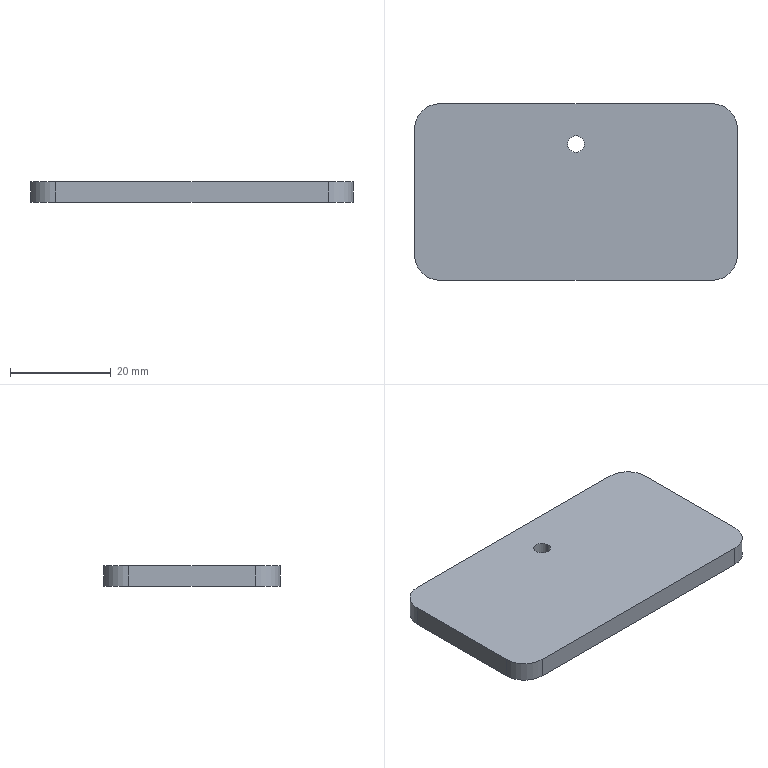Part | STEP file | 001-006-Pre-insertion mechanism slider connecting plate | 1 solid | 12 faces | box 64 x 35 x 4 mm | volume 8840 mm3 | cylinder 6 | plane 6 | commonest cylinder face diameters 10 x4 3.3 x2
STEP:
#1=CARTESIAN_POINT('',(0.,0.,0.));
#2=DIRECTION('',(0.,0.,1.));
#3=DIRECTION('',(1.,0.,0.));
#4=AXIS2_PLACEMENT_3D('',#1,#2,#3);
#5=CARTESIAN_POINT('',(1.65,9.5,0.));
#6=VERTEX_POINT('',#5);
#7=CARTESIAN_POINT('',(1.65,9.5,4.));
#8=VERTEX_POINT('',#7);
#9=CARTESIAN_POINT('',(1.65,9.5,4.));
#10=DIRECTION('',(0.,0.,1.));
#11=VECTOR('',#10,1.);
#12=LINE('',#9,#11);
#13=CARTESIAN_POINT('',(0.,9.5,4.));
#14=DIRECTION('',(0.,0.,1.));
#15=DIRECTION('',(1.,0.,0.));
#16=AXIS2_PLACEMENT_3D('',#13,#14,#15);
#17=CYLINDRICAL_SURFACE('',#16,1.65);
#18=CARTESIAN_POINT('',(6.283,0.));
#19=DIRECTION('',(0.,1.));
#20=VECTOR('',#19,1.);
#21=LINE('',#18,#20);
#22=(GEOMETRIC_REPRESENTATION_CONTEXT(2)PARAMETRIC_REPRESENTATION_CONTEXT()REPRESENTATION_CONTEXT('',''));
#23=DEFINITIONAL_REPRESENTATION('',(#21),#22);
#24=PCURVE('',#17,#23);
#25=CARTESIAN_POINT('',(0.,9.5,4.));
#26=DIRECTION('',(0.,0.,1.));
#27=DIRECTION('',(1.,0.,0.));
#28=AXIS2_PLACEMENT_3D('',#25,#26,#27);
#29=CYLINDRICAL_SURFACE('',#28,1.65);
#30=CARTESIAN_POINT('',(0.,0.));
#31=DIRECTION('',(0.,1.));
#32=VECTOR('',#31,1.);
#33=LINE('',#30,#32);
#34=(GEOMETRIC_REPRESENTATION_CONTEXT(2)PARAMETRIC_REPRESENTATION_CONTEXT()REPRESENTATION_CONTEXT('',''));
#35=DEFINITIONAL_REPRESENTATION('',(#33),#34);
#36=PCURVE('',#29,#35);
#37=SURFACE_CURVE('',#12,(#24,#36),.PCURVE_S1.);
#38=EDGE_CURVE('',#6,#8,#37,.T.);
#39=ORIENTED_EDGE('',*,*,#38,.T.);
#40=CARTESIAN_POINT('',(-1.65,9.5,4.));
#41=VERTEX_POINT('',#40);
#42=CARTESIAN_POINT('',(0.,9.5,4.));
#43=DIRECTION('',(0.,0.,1.));
#44=DIRECTION('',(1.,0.,0.));
#45=AXIS2_PLACEMENT_3D('',#42,#43,#44);
#46=CIRCLE('',#45,1.65);
#47=CARTESIAN_POINT('',(0.,0.));
#48=DIRECTION('',(1.,0.));
#49=VECTOR('',#48,1.);
#50=LINE('',#47,#49);
#51=(GEOMETRIC_REPRESENTATION_CONTEXT(2)PARAMETRIC_REPRESENTATION_CONTEXT()REPRESENTATION_CONTEXT('',''));
#52=DEFINITIONAL_REPRESENTATION('',(#50),#51);
#53=PCURVE('',#17,#52);
#54=CARTESIAN_POINT('',(0.,0.,4.));
#55=DIRECTION('',(0.,0.,-1.));
#56=DIRECTION('',(-1.,0.,0.));
#57=AXIS2_PLACEMENT_3D('',#54,#55,#56);
#58=PLANE('',#57);
#59=CARTESIAN_POINT('',(-1.65,9.5));
#60=CARTESIAN_POINT('',(-1.65,12.358));
#61=CARTESIAN_POINT('',(0.825,10.929));
#62=CARTESIAN_POINT('',(3.3,9.5));
#63=CARTESIAN_POINT('',(0.825,8.071));
#64=CARTESIAN_POINT('',(-1.65,6.642));
#65=CARTESIAN_POINT('',(-1.65,9.5));
#66=(BOUNDED_CURVE()B_SPLINE_CURVE(2,(#59,#60,#61,#62,#63,#64,#65),.UNSPECIFIED.,.T.,.F.)B_SPLINE_CURVE_WITH_KNOTS((1,2,2,2,2,1),(-2.094,0.,2.094,4.189,6.283,8.378),.UNSPECIFIED.)CURVE()GEOMETRIC_REPRESENTATION_ITEM()RATIONAL_B_SPLINE_CURVE((1.,0.5,1.,0.5,1.,0.5,1.))REPRESENTATION_ITEM(''));
#67=(GEOMETRIC_REPRESENTATION_CONTEXT(2)PARAMETRIC_REPRESENTATION_CONTEXT()REPRESENTATION_CONTEXT('',''));
#68=DEFINITIONAL_REPRESENTATION('',(#66),#67);
#69=PCURVE('',#58,#68);
#70=SURFACE_CURVE('',#46,(#53,#69),.PCURVE_S1.);
#71=EDGE_CURVE('',#41,#8,#70,.T.);
#72=ORIENTED_EDGE('',*,*,#71,.F.);
#73=CARTESIAN_POINT('',(-1.65,9.5,0.));
#74=VERTEX_POINT('',#73);
#75=CARTESIAN_POINT('',(-1.65,9.5,4.));
#76=DIRECTION('',(0.,0.,1.));
#77=VECTOR('',#76,1.);
#78=LINE('',#75,#77);
#79=CARTESIAN_POINT('',(3.142,0.));
#80=DIRECTION('',(0.,1.));
#81=VECTOR('',#80,1.);
#82=LINE('',#79,#81);
#83=(GEOMETRIC_REPRESENTATION_CONTEXT(2)PARAMETRIC_REPRESENTATION_CONTEXT()REPRESENTATION_CONTEXT('',''));
#84=DEFINITIONAL_REPRESENTATION('',(#82),#83);
#85=PCURVE('',#17,#84);
#86=CARTESIAN_POINT('',(3.142,0.));
#87=DIRECTION('',(0.,1.));
#88=VECTOR('',#87,1.);
#89=LINE('',#86,#88);
#90=(GEOMETRIC_REPRESENTATION_CONTEXT(2)PARAMETRIC_REPRESENTATION_CONTEXT()REPRESENTATION_CONTEXT('',''));
#91=DEFINITIONAL_REPRESENTATION('',(#89),#90);
#92=PCURVE('',#29,#91);
#93=SURFACE_CURVE('',#78,(#85,#92),.PCURVE_S1.);
#94=EDGE_CURVE('',#74,#41,#93,.T.);
#95=ORIENTED_EDGE('',*,*,#94,.F.);
#96=CARTESIAN_POINT('',(0.,9.5,0.));
#97=DIRECTION('',(0.,0.,1.));
#98=DIRECTION('',(1.,0.,0.));
#99=AXIS2_PLACEMENT_3D('',#96,#97,#98);
#100=CIRCLE('',#99,1.65);
#101=CARTESIAN_POINT('',(0.,-4.));
#102=DIRECTION('',(1.,0.));
#103=VECTOR('',#102,1.);
#104=LINE('',#101,#103);
#105=(GEOMETRIC_REPRESENTATION_CONTEXT(2)PARAMETRIC_REPRESENTATION_CONTEXT()REPRESENTATION_CONTEXT('',''));
#106=DEFINITIONAL_REPRESENTATION('',(#104),#105);
#107=PCURVE('',#17,#106);
#108=CARTESIAN_POINT('',(0.,0.,0.));
#109=DIRECTION('',(0.,0.,-1.));
#110=DIRECTION('',(-1.,0.,0.));
#111=AXIS2_PLACEMENT_3D('',#108,#109,#110);
#112=PLANE('',#111);
#113=CARTESIAN_POINT('',(-1.65,9.5));
#114=CARTESIAN_POINT('',(-1.65,12.358));
#115=CARTESIAN_POINT('',(0.825,10.929));
#116=CARTESIAN_POINT('',(3.3,9.5));
#117=CARTESIAN_POINT('',(0.825,8.071));
#118=CARTESIAN_POINT('',(-1.65,6.642));
#119=CARTESIAN_POINT('',(-1.65,9.5));
#120=(BOUNDED_CURVE()B_SPLINE_CURVE(2,(#113,#114,#115,#116,#117,#118,#119),.UNSPECIFIED.,.T.,.F.)B_SPLINE_CURVE_WITH_KNOTS((1,2,2,2,2,1),(-2.094,0.,2.094,4.189,6.283,8.378),.UNSPECIFIED.)CURVE()GEOMETRIC_REPRESENTATION_ITEM()RATIONAL_B_SPLINE_CURVE((1.,0.5,1.,0.5,1.,0.5,1.))REPRESENTATION_ITEM(''));
#121=(GEOMETRIC_REPRESENTATION_CONTEXT(2)PARAMETRIC_REPRESENTATION_CONTEXT()REPRESENTATION_CONTEXT('',''));
#122=DEFINITIONAL_REPRESENTATION('',(#120),#121);
#123=PCURVE('',#112,#122);
#124=SURFACE_CURVE('',#100,(#107,#123),.PCURVE_S1.);
#125=EDGE_CURVE('',#74,#6,#124,.T.);
#126=ORIENTED_EDGE('',*,*,#125,.T.);
#127=EDGE_LOOP('',(#39,#72,#95,#126));
#128=FACE_BOUND('',#127,.F.);
#129=ADVANCED_FACE('',(#128),#17,.F.);
#130=CARTESIAN_POINT('',(32.,-12.5,4.));
#131=VERTEX_POINT('',#130);
#132=CARTESIAN_POINT('',(32.,12.5,4.));
#133=VERTEX_POINT('',#132);
#134=CARTESIAN_POINT('',(32.,-17.5,4.));
#135=DIRECTION('',(0.,1.,0.));
#136=VECTOR('',#135,1.);
#137=LINE('',#134,#136);
#138=CARTESIAN_POINT('',(32.,-17.5,4.));
#139=DIRECTION('',(-1.,0.,0.));
#140=DIRECTION('',(0.,-1.,0.));
#141=AXIS2_PLACEMENT_3D('',#138,#139,#140);
#142=PLANE('',#141);
#143=CARTESIAN_POINT('',(0.,0.));
#144=DIRECTION('',(-1.,0.));
#145=VECTOR('',#144,1.);
#146=LINE('',#143,#145);
#147=(GEOMETRIC_REPRESENTATION_CONTEXT(2)PARAMETRIC_REPRESENTATION_CONTEXT()REPRESENTATION_CONTEXT('',''));
#148=DEFINITIONAL_REPRESENTATION('',(#146),#147);
#149=PCURVE('',#142,#148);
#150=CARTESIAN_POINT('',(-32.,-17.5));
#151=DIRECTION('',(0.,1.));
#152=VECTOR('',#151,1.);
#153=LINE('',#150,#152);
#154=(GEOMETRIC_REPRESENTATION_CONTEXT(2)PARAMETRIC_REPRESENTATION_CONTEXT()REPRESENTATION_CONTEXT('',''));
#155=DEFINITIONAL_REPRESENTATION('',(#153),#154);
#156=PCURVE('',#58,#155);
#157=SURFACE_CURVE('',#137,(#149,#156),.PCURVE_S1.);
#158=EDGE_CURVE('',#131,#133,#157,.T.);
#159=ORIENTED_EDGE('',*,*,#158,.F.);
#160=CARTESIAN_POINT('',(32.,-12.5,0.));
#161=VERTEX_POINT('',#160);
#162=CARTESIAN_POINT('',(32.,-12.5,4.));
#163=DIRECTION('',(0.,0.,-1.));
#164=VECTOR('',#163,1.);
#165=LINE('',#162,#164);
#166=CARTESIAN_POINT('',(-5.,0.));
#167=DIRECTION('',(0.,-1.));
#168=VECTOR('',#167,1.);
#169=LINE('',#166,#168);
#170=(GEOMETRIC_REPRESENTATION_CONTEXT(2)PARAMETRIC_REPRESENTATION_CONTEXT()REPRESENTATION_CONTEXT('',''));
#171=DEFINITIONAL_REPRESENTATION('',(#169),#170);
#172=PCURVE('',#142,#171);
#173=CARTESIAN_POINT('',(27.,-12.5,4.));
#174=DIRECTION('',(0.,0.,-1.));
#175=DIRECTION('',(-1.,0.,0.));
#176=AXIS2_PLACEMENT_3D('',#173,#174,#175);
#177=CYLINDRICAL_SURFACE('',#176,5.);
#178=CARTESIAN_POINT('',(3.142,0.));
#179=DIRECTION('',(0.,1.));
#180=VECTOR('',#179,1.);
#181=LINE('',#178,#180);
#182=(GEOMETRIC_REPRESENTATION_CONTEXT(2)PARAMETRIC_REPRESENTATION_CONTEXT()REPRESENTATION_CONTEXT('',''));
#183=DEFINITIONAL_REPRESENTATION('',(#181),#182);
#184=PCURVE('',#177,#183);
#185=SURFACE_CURVE('',#165,(#172,#184),.PCURVE_S1.);
#186=EDGE_CURVE('',#131,#161,#185,.T.);
#187=ORIENTED_EDGE('',*,*,#186,.T.);
#188=CARTESIAN_POINT('',(32.,12.5,0.));
#189=VERTEX_POINT('',#188);
#190=CARTESIAN_POINT('',(32.,-17.5,0.));
#191=DIRECTION('',(0.,1.,0.));
#192=VECTOR('',#191,1.);
#193=LINE('',#190,#192);
#194=CARTESIAN_POINT('',(0.,-4.));
#195=DIRECTION('',(-1.,0.));
#196=VECTOR('',#195,1.);
#197=LINE('',#194,#196);
#198=(GEOMETRIC_REPRESENTATION_CONTEXT(2)PARAMETRIC_REPRESENTATION_CONTEXT()REPRESENTATION_CONTEXT('',''));
#199=DEFINITIONAL_REPRESENTATION('',(#197),#198);
#200=PCURVE('',#142,#199);
#201=CARTESIAN_POINT('',(-32.,-17.5));
#202=DIRECTION('',(0.,1.));
#203=VECTOR('',#202,1.);
#204=LINE('',#201,#203);
#205=(GEOMETRIC_REPRESENTATION_CONTEXT(2)PARAMETRIC_REPRESENTATION_CONTEXT()REPRESENTATION_CONTEXT('',''));
#206=DEFINITIONAL_REPRESENTATION('',(#204),#205);
#207=PCURVE('',#112,#206);
#208=SURFACE_CURVE('',#193,(#200,#207),.PCURVE_S1.);
#209=EDGE_CURVE('',#161,#189,#208,.T.);
#210=ORIENTED_EDGE('',*,*,#209,.T.);
#211=CARTESIAN_POINT('',(32.,12.5,4.));
#212=DIRECTION('',(0.,0.,1.));
#213=VECTOR('',#212,1.);
#214=LINE('',#211,#213);
#215=CARTESIAN_POINT('',(-30.,0.));
#216=DIRECTION('',(0.,1.));
#217=VECTOR('',#216,1.);
#218=LINE('',#215,#217);
#219=(GEOMETRIC_REPRESENTATION_CONTEXT(2)PARAMETRIC_REPRESENTATION_CONTEXT()REPRESENTATION_CONTEXT('',''));
#220=DEFINITIONAL_REPRESENTATION('',(#218),#219);
#221=PCURVE('',#142,#220);
#222=CARTESIAN_POINT('',(27.,12.5,4.));
#223=DIRECTION('',(0.,0.,-1.));
#224=DIRECTION('',(-1.,0.,0.));
#225=AXIS2_PLACEMENT_3D('',#222,#223,#224);
#226=CYLINDRICAL_SURFACE('',#225,5.);
#227=CARTESIAN_POINT('',(3.142,0.));
#228=DIRECTION('',(0.,-1.));
#229=VECTOR('',#228,1.);
#230=LINE('',#227,#229);
#231=(GEOMETRIC_REPRESENTATION_CONTEXT(2)PARAMETRIC_REPRESENTATION_CONTEXT()REPRESENTATION_CONTEXT('',''));
#232=DEFINITIONAL_REPRESENTATION('',(#230),#231);
#233=PCURVE('',#226,#232);
#234=SURFACE_CURVE('',#214,(#221,#233),.PCURVE_S1.);
#235=EDGE_CURVE('',#189,#133,#234,.T.);
#236=ORIENTED_EDGE('',*,*,#235,.T.);
#237=EDGE_LOOP('',(#159,#187,#210,#236));
#238=FACE_BOUND('',#237,.T.);
#239=ADVANCED_FACE('',(#238),#142,.F.);
#240=CARTESIAN_POINT('',(27.,17.5,0.));
#241=VERTEX_POINT('',#240);
#242=CARTESIAN_POINT('',(-27.,17.5,0.));
#243=VERTEX_POINT('',#242);
#244=CARTESIAN_POINT('',(-32.,17.5,0.));
#245=DIRECTION('',(-1.,0.,0.));
#246=VECTOR('',#245,1.);
#247=LINE('',#244,#246);
#248=CARTESIAN_POINT('',(-32.,17.5,4.));
#249=DIRECTION('',(0.,-1.,0.));
#250=DIRECTION('',(1.,0.,0.));
#251=AXIS2_PLACEMENT_3D('',#248,#249,#250);
#252=PLANE('',#251);
#253=CARTESIAN_POINT('',(0.,-4.));
#254=DIRECTION('',(-1.,0.));
#255=VECTOR('',#254,1.);
#256=LINE('',#253,#255);
#257=(GEOMETRIC_REPRESENTATION_CONTEXT(2)PARAMETRIC_REPRESENTATION_CONTEXT()REPRESENTATION_CONTEXT('',''));
#258=DEFINITIONAL_REPRESENTATION('',(#256),#257);
#259=PCURVE('',#252,#258);
#260=CARTESIAN_POINT('',(32.,17.5));
#261=DIRECTION('',(1.,0.));
#262=VECTOR('',#261,1.);
#263=LINE('',#260,#262);
#264=(GEOMETRIC_REPRESENTATION_CONTEXT(2)PARAMETRIC_REPRESENTATION_CONTEXT()REPRESENTATION_CONTEXT('',''));
#265=DEFINITIONAL_REPRESENTATION('',(#263),#264);
#266=PCURVE('',#112,#265);
#267=SURFACE_CURVE('',#247,(#259,#266),.PCURVE_S1.);
#268=EDGE_CURVE('',#241,#243,#267,.T.);
#269=ORIENTED_EDGE('',*,*,#268,.T.);
#270=CARTESIAN_POINT('',(-27.,17.5,4.));
#271=VERTEX_POINT('',#270);
#272=CARTESIAN_POINT('',(-27.,17.5,4.));
#273=DIRECTION('',(0.,0.,1.));
#274=VECTOR('',#273,1.);
#275=LINE('',#272,#274);
#276=CARTESIAN_POINT('',(5.,0.));
#277=DIRECTION('',(0.,1.));
#278=VECTOR('',#277,1.);
#279=LINE('',#276,#278);
#280=(GEOMETRIC_REPRESENTATION_CONTEXT(2)PARAMETRIC_REPRESENTATION_CONTEXT()REPRESENTATION_CONTEXT('',''));
#281=DEFINITIONAL_REPRESENTATION('',(#279),#280);
#282=PCURVE('',#252,#281);
#283=CARTESIAN_POINT('',(-27.,12.5,4.));
#284=DIRECTION('',(0.,0.,-1.));
#285=DIRECTION('',(-1.,0.,0.));
#286=AXIS2_PLACEMENT_3D('',#283,#284,#285);
#287=CYLINDRICAL_SURFACE('',#286,5.);
#288=CARTESIAN_POINT('',(1.571,0.));
#289=DIRECTION('',(0.,-1.));
#290=VECTOR('',#289,1.);
#291=LINE('',#288,#290);
#292=(GEOMETRIC_REPRESENTATION_CONTEXT(2)PARAMETRIC_REPRESENTATION_CONTEXT()REPRESENTATION_CONTEXT('',''));
#293=DEFINITIONAL_REPRESENTATION('',(#291),#292);
#294=PCURVE('',#287,#293);
#295=SURFACE_CURVE('',#275,(#282,#294),.PCURVE_S1.);
#296=EDGE_CURVE('',#243,#271,#295,.T.);
#297=ORIENTED_EDGE('',*,*,#296,.T.);
#298=CARTESIAN_POINT('',(27.,17.5,4.));
#299=VERTEX_POINT('',#298);
#300=CARTESIAN_POINT('',(-32.,17.5,4.));
#301=DIRECTION('',(-1.,0.,0.));
#302=VECTOR('',#301,1.);
#303=LINE('',#300,#302);
#304=CARTESIAN_POINT('',(0.,0.));
#305=DIRECTION('',(-1.,0.));
#306=VECTOR('',#305,1.);
#307=LINE('',#304,#306);
#308=(GEOMETRIC_REPRESENTATION_CONTEXT(2)PARAMETRIC_REPRESENTATION_CONTEXT()REPRESENTATION_CONTEXT('',''));
#309=DEFINITIONAL_REPRESENTATION('',(#307),#308);
#310=PCURVE('',#252,#309);
#311=CARTESIAN_POINT('',(32.,17.5));
#312=DIRECTION('',(1.,0.));
#313=VECTOR('',#312,1.);
#314=LINE('',#311,#313);
#315=(GEOMETRIC_REPRESENTATION_CONTEXT(2)PARAMETRIC_REPRESENTATION_CONTEXT()REPRESENTATION_CONTEXT('',''));
#316=DEFINITIONAL_REPRESENTATION('',(#314),#315);
#317=PCURVE('',#58,#316);
#318=SURFACE_CURVE('',#303,(#310,#317),.PCURVE_S1.);
#319=EDGE_CURVE('',#299,#271,#318,.T.);
#320=ORIENTED_EDGE('',*,*,#319,.F.);
#321=CARTESIAN_POINT('',(27.,17.5,4.));
#322=DIRECTION('',(0.,0.,-1.));
#323=VECTOR('',#322,1.);
#324=LINE('',#321,#323);
#325=CARTESIAN_POINT('',(59.,0.));
#326=DIRECTION('',(0.,-1.));
#327=VECTOR('',#326,1.);
#328=LINE('',#325,#327);
#329=(GEOMETRIC_REPRESENTATION_CONTEXT(2)PARAMETRIC_REPRESENTATION_CONTEXT()REPRESENTATION_CONTEXT('',''));
#330=DEFINITIONAL_REPRESENTATION('',(#328),#329);
#331=PCURVE('',#252,#330);
#332=CARTESIAN_POINT('',(1.571,0.));
#333=DIRECTION('',(0.,1.));
#334=VECTOR('',#333,1.);
#335=LINE('',#332,#334);
#336=(GEOMETRIC_REPRESENTATION_CONTEXT(2)PARAMETRIC_REPRESENTATION_CONTEXT()REPRESENTATION_CONTEXT('',''));
#337=DEFINITIONAL_REPRESENTATION('',(#335),#336);
#338=PCURVE('',#226,#337);
#339=SURFACE_CURVE('',#324,(#331,#338),.PCURVE_S1.);
#340=EDGE_CURVE('',#299,#241,#339,.T.);
#341=ORIENTED_EDGE('',*,*,#340,.T.);
#342=EDGE_LOOP('',(#269,#297,#320,#341));
#343=FACE_BOUND('',#342,.T.);
#344=ADVANCED_FACE('',(#343),#252,.F.);
#345=CARTESIAN_POINT('',(-32.,12.5,0.));
#346=VERTEX_POINT('',#345);
#347=CARTESIAN_POINT('',(-32.,-12.5,0.));
#348=VERTEX_POINT('',#347);
#349=CARTESIAN_POINT('',(-32.,-17.5,0.));
#350=DIRECTION('',(0.,-1.,0.));
#351=VECTOR('',#350,1.);
#352=LINE('',#349,#351);
#353=CARTESIAN_POINT('',(-32.,-17.5,4.));
#354=DIRECTION('',(1.,0.,0.));
#355=DIRECTION('',(0.,1.,0.));
#356=AXIS2_PLACEMENT_3D('',#353,#354,#355);
#357=PLANE('',#356);
#358=CARTESIAN_POINT('',(0.,-4.));
#359=DIRECTION('',(-1.,0.));
#360=VECTOR('',#359,1.);
#361=LINE('',#358,#360);
#362=(GEOMETRIC_REPRESENTATION_CONTEXT(2)PARAMETRIC_REPRESENTATION_CONTEXT()REPRESENTATION_CONTEXT('',''));
#363=DEFINITIONAL_REPRESENTATION('',(#361),#362);
#364=PCURVE('',#357,#363);
#365=CARTESIAN_POINT('',(32.,-17.5));
#366=DIRECTION('',(0.,-1.));
#367=VECTOR('',#366,1.);
#368=LINE('',#365,#367);
#369=(GEOMETRIC_REPRESENTATION_CONTEXT(2)PARAMETRIC_REPRESENTATION_CONTEXT()REPRESENTATION_CONTEXT('',''));
#370=DEFINITIONAL_REPRESENTATION('',(#368),#369);
#371=PCURVE('',#112,#370);
#372=SURFACE_CURVE('',#352,(#364,#371),.PCURVE_S1.);
#373=EDGE_CURVE('',#346,#348,#372,.T.);
#374=ORIENTED_EDGE('',*,*,#373,.T.);
#375=CARTESIAN_POINT('',(-32.,-12.5,4.));
#376=VERTEX_POINT('',#375);
#377=CARTESIAN_POINT('',(-32.,-12.5,4.));
#378=DIRECTION('',(0.,0.,1.));
#379=VECTOR('',#378,1.);
#380=LINE('',#377,#379);
#381=CARTESIAN_POINT('',(5.,0.));
#382=DIRECTION('',(0.,1.));
#383=VECTOR('',#382,1.);
#384=LINE('',#381,#383);
#385=(GEOMETRIC_REPRESENTATION_CONTEXT(2)PARAMETRIC_REPRESENTATION_CONTEXT()REPRESENTATION_CONTEXT('',''));
#386=DEFINITIONAL_REPRESENTATION('',(#384),#385);
#387=PCURVE('',#357,#386);
#388=CARTESIAN_POINT('',(-27.,-12.5,4.));
#389=DIRECTION('',(0.,0.,-1.));
#390=DIRECTION('',(-1.,0.,0.));
#391=AXIS2_PLACEMENT_3D('',#388,#389,#390);
#392=CYLINDRICAL_SURFACE('',#391,5.);
#393=CARTESIAN_POINT('',(6.283,0.));
#394=DIRECTION('',(0.,-1.));
#395=VECTOR('',#394,1.);
#396=LINE('',#393,#395);
#397=(GEOMETRIC_REPRESENTATION_CONTEXT(2)PARAMETRIC_REPRESENTATION_CONTEXT()REPRESENTATION_CONTEXT('',''));
#398=DEFINITIONAL_REPRESENTATION('',(#396),#397);
#399=PCURVE('',#392,#398);
#400=SURFACE_CURVE('',#380,(#387,#399),.PCURVE_S1.);
#401=EDGE_CURVE('',#348,#376,#400,.T.);
#402=ORIENTED_EDGE('',*,*,#401,.T.);
#403=CARTESIAN_POINT('',(-32.,12.5,4.));
#404=VERTEX_POINT('',#403);
#405=CARTESIAN_POINT('',(-32.,-17.5,4.));
#406=DIRECTION('',(0.,-1.,0.));
#407=VECTOR('',#406,1.);
#408=LINE('',#405,#407);
#409=CARTESIAN_POINT('',(0.,0.));
#410=DIRECTION('',(-1.,0.));
#411=VECTOR('',#410,1.);
#412=LINE('',#409,#411);
#413=(GEOMETRIC_REPRESENTATION_CONTEXT(2)PARAMETRIC_REPRESENTATION_CONTEXT()REPRESENTATION_CONTEXT('',''));
#414=DEFINITIONAL_REPRESENTATION('',(#412),#413);
#415=PCURVE('',#357,#414);
#416=CARTESIAN_POINT('',(32.,-17.5));
#417=DIRECTION('',(0.,-1.));
#418=VECTOR('',#417,1.);
#419=LINE('',#416,#418);
#420=(GEOMETRIC_REPRESENTATION_CONTEXT(2)PARAMETRIC_REPRESENTATION_CONTEXT()REPRESENTATION_CONTEXT('',''));
#421=DEFINITIONAL_REPRESENTATION('',(#419),#420);
#422=PCURVE('',#58,#421);
#423=SURFACE_CURVE('',#408,(#415,#422),.PCURVE_S1.);
#424=EDGE_CURVE('',#404,#376,#423,.T.);
#425=ORIENTED_EDGE('',*,*,#424,.F.);
#426=CARTESIAN_POINT('',(-32.,12.5,4.));
#427=DIRECTION('',(0.,0.,-1.));
#428=VECTOR('',#427,1.);
#429=LINE('',#426,#428);
#430=CARTESIAN_POINT('',(30.,0.));
#431=DIRECTION('',(0.,-1.));
#432=VECTOR('',#431,1.);
#433=LINE('',#430,#432);
#434=(GEOMETRIC_REPRESENTATION_CONTEXT(2)PARAMETRIC_REPRESENTATION_CONTEXT()REPRESENTATION_CONTEXT('',''));
#435=DEFINITIONAL_REPRESENTATION('',(#433),#434);
#436=PCURVE('',#357,#435);
#437=CARTESIAN_POINT('',(0.,0.));
#438=DIRECTION('',(0.,1.));
#439=VECTOR('',#438,1.);
#440=LINE('',#437,#439);
#441=(GEOMETRIC_REPRESENTATION_CONTEXT(2)PARAMETRIC_REPRESENTATION_CONTEXT()REPRESENTATION_CONTEXT('',''));
#442=DEFINITIONAL_REPRESENTATION('',(#440),#441);
#443=PCURVE('',#287,#442);
#444=SURFACE_CURVE('',#429,(#436,#443),.PCURVE_S1.);
#445=EDGE_CURVE('',#404,#346,#444,.T.);
#446=ORIENTED_EDGE('',*,*,#445,.T.);
#447=EDGE_LOOP('',(#374,#402,#425,#446));
#448=FACE_BOUND('',#447,.T.);
#449=ADVANCED_FACE('',(#448),#357,.F.);
#450=CARTESIAN_POINT('',(-27.,-17.5,0.));
#451=VERTEX_POINT('',#450);
#452=CARTESIAN_POINT('',(27.,-17.5,0.));
#453=VERTEX_POINT('',#452);
#454=CARTESIAN_POINT('',(-32.,-17.5,0.));
#455=DIRECTION('',(1.,0.,0.));
#456=VECTOR('',#455,1.);
#457=LINE('',#454,#456);
#458=CARTESIAN_POINT('',(-32.,-17.5,4.));
#459=DIRECTION('',(0.,1.,0.));
#460=DIRECTION('',(-1.,0.,0.));
#461=AXIS2_PLACEMENT_3D('',#458,#459,#460);
#462=PLANE('',#461);
#463=CARTESIAN_POINT('',(0.,-4.));
#464=DIRECTION('',(-1.,0.));
#465=VECTOR('',#464,1.);
#466=LINE('',#463,#465);
#467=(GEOMETRIC_REPRESENTATION_CONTEXT(2)PARAMETRIC_REPRESENTATION_CONTEXT()REPRESENTATION_CONTEXT('',''));
#468=DEFINITIONAL_REPRESENTATION('',(#466),#467);
#469=PCURVE('',#462,#468);
#470=CARTESIAN_POINT('',(32.,-17.5));
#471=DIRECTION('',(-1.,0.));
#472=VECTOR('',#471,1.);
#473=LINE('',#470,#472);
#474=(GEOMETRIC_REPRESENTATION_CONTEXT(2)PARAMETRIC_REPRESENTATION_CONTEXT()REPRESENTATION_CONTEXT('',''));
#475=DEFINITIONAL_REPRESENTATION('',(#473),#474);
#476=PCURVE('',#112,#475);
#477=SURFACE_CURVE('',#457,(#469,#476),.PCURVE_S1.);
#478=EDGE_CURVE('',#451,#453,#477,.T.);
#479=ORIENTED_EDGE('',*,*,#478,.T.);
#480=CARTESIAN_POINT('',(27.,-17.5,4.));
#481=VERTEX_POINT('',#480);
#482=CARTESIAN_POINT('',(27.,-17.5,4.));
#483=DIRECTION('',(0.,0.,1.));
#484=VECTOR('',#483,1.);
#485=LINE('',#482,#484);
#486=CARTESIAN_POINT('',(-59.,0.));
#487=DIRECTION('',(0.,1.));
#488=VECTOR('',#487,1.);
#489=LINE('',#486,#488);
#490=(GEOMETRIC_REPRESENTATION_CONTEXT(2)PARAMETRIC_REPRESENTATION_CONTEXT()REPRESENTATION_CONTEXT('',''));
#491=DEFINITIONAL_REPRESENTATION('',(#489),#490);
#492=PCURVE('',#462,#491);
#493=CARTESIAN_POINT('',(4.712,0.));
#494=DIRECTION('',(0.,-1.));
#495=VECTOR('',#494,1.);
#496=LINE('',#493,#495);
#497=(GEOMETRIC_REPRESENTATION_CONTEXT(2)PARAMETRIC_REPRESENTATION_CONTEXT()REPRESENTATION_CONTEXT('',''));
#498=DEFINITIONAL_REPRESENTATION('',(#496),#497);
#499=PCURVE('',#177,#498);
#500=SURFACE_CURVE('',#485,(#492,#499),.PCURVE_S1.);
#501=EDGE_CURVE('',#453,#481,#500,.T.);
#502=ORIENTED_EDGE('',*,*,#501,.T.);
#503=CARTESIAN_POINT('',(-27.,-17.5,4.));
#504=VERTEX_POINT('',#503);
#505=CARTESIAN_POINT('',(-32.,-17.5,4.));
#506=DIRECTION('',(1.,0.,0.));
#507=VECTOR('',#506,1.);
#508=LINE('',#505,#507);
#509=CARTESIAN_POINT('',(0.,0.));
#510=DIRECTION('',(-1.,0.));
#511=VECTOR('',#510,1.);
#512=LINE('',#509,#511);
#513=(GEOMETRIC_REPRESENTATION_CONTEXT(2)PARAMETRIC_REPRESENTATION_CONTEXT()REPRESENTATION_CONTEXT('',''));
#514=DEFINITIONAL_REPRESENTATION('',(#512),#513);
#515=PCURVE('',#462,#514);
#516=CARTESIAN_POINT('',(32.,-17.5));
#517=DIRECTION('',(-1.,0.));
#518=VECTOR('',#517,1.);
#519=LINE('',#516,#518);
#520=(GEOMETRIC_REPRESENTATION_CONTEXT(2)PARAMETRIC_REPRESENTATION_CONTEXT()REPRESENTATION_CONTEXT('',''));
#521=DEFINITIONAL_REPRESENTATION('',(#519),#520);
#522=PCURVE('',#58,#521);
#523=SURFACE_CURVE('',#508,(#515,#522),.PCURVE_S1.);
#524=EDGE_CURVE('',#504,#481,#523,.T.);
#525=ORIENTED_EDGE('',*,*,#524,.F.);
#526=CARTESIAN_POINT('',(-27.,-17.5,4.));
#527=DIRECTION('',(0.,0.,-1.));
#528=VECTOR('',#527,1.);
#529=LINE('',#526,#528);
#530=CARTESIAN_POINT('',(-5.,0.));
#531=DIRECTION('',(0.,-1.));
#532=VECTOR('',#531,1.);
#533=LINE('',#530,#532);
#534=(GEOMETRIC_REPRESENTATION_CONTEXT(2)PARAMETRIC_REPRESENTATION_CONTEXT()REPRESENTATION_CONTEXT('',''));
#535=DEFINITIONAL_REPRESENTATION('',(#533),#534);
#536=PCURVE('',#462,#535);
#537=CARTESIAN_POINT('',(4.712,0.));
#538=DIRECTION('',(0.,1.));
#539=VECTOR('',#538,1.);
#540=LINE('',#537,#539);
#541=(GEOMETRIC_REPRESENTATION_CONTEXT(2)PARAMETRIC_REPRESENTATION_CONTEXT()REPRESENTATION_CONTEXT('',''));
#542=DEFINITIONAL_REPRESENTATION('',(#540),#541);
#543=PCURVE('',#392,#542);
#544=SURFACE_CURVE('',#529,(#536,#543),.PCURVE_S1.);
#545=EDGE_CURVE('',#504,#451,#544,.T.);
#546=ORIENTED_EDGE('',*,*,#545,.T.);
#547=EDGE_LOOP('',(#479,#502,#525,#546));
#548=FACE_BOUND('',#547,.T.);
#549=ADVANCED_FACE('',(#548),#462,.F.);
#550=CARTESIAN_POINT('',(0.,9.5,4.));
#551=DIRECTION('',(0.,0.,1.));
#552=DIRECTION('',(1.,0.,0.));
#553=AXIS2_PLACEMENT_3D('',#550,#551,#552);
#554=CIRCLE('',#553,1.65);
#555=CARTESIAN_POINT('',(-1.65,9.5));
#556=CARTESIAN_POINT('',(-1.65,12.358));
#557=CARTESIAN_POINT('',(0.825,10.929));
#558=CARTESIAN_POINT('',(3.3,9.5));
#559=CARTESIAN_POINT('',(0.825,8.071));
#560=CARTESIAN_POINT('',(-1.65,6.642));
#561=CARTESIAN_POINT('',(-1.65,9.5));
#562=(BOUNDED_CURVE()B_SPLINE_CURVE(2,(#555,#556,#557,#558,#559,#560,#561),.UNSPECIFIED.,.T.,.F.)B_SPLINE_CURVE_WITH_KNOTS((1,2,2,2,2,1),(-2.094,0.,2.094,4.189,6.283,8.378),.UNSPECIFIED.)CURVE()GEOMETRIC_REPRESENTATION_ITEM()RATIONAL_B_SPLINE_CURVE((1.,0.5,1.,0.5,1.,0.5,1.))REPRESENTATION_ITEM(''));
#563=(GEOMETRIC_REPRESENTATION_CONTEXT(2)PARAMETRIC_REPRESENTATION_CONTEXT()REPRESENTATION_CONTEXT('',''));
#564=DEFINITIONAL_REPRESENTATION('',(#562),#563);
#565=PCURVE('',#58,#564);
#566=CARTESIAN_POINT('',(0.,0.));
#567=DIRECTION('',(1.,0.));
#568=VECTOR('',#567,1.);
#569=LINE('',#566,#568);
#570=(GEOMETRIC_REPRESENTATION_CONTEXT(2)PARAMETRIC_REPRESENTATION_CONTEXT()REPRESENTATION_CONTEXT('',''));
#571=DEFINITIONAL_REPRESENTATION('',(#569),#570);
#572=PCURVE('',#29,#571);
#573=SURFACE_CURVE('',#554,(#565,#572),.PCURVE_S1.);
#574=EDGE_CURVE('',#8,#41,#573,.T.);
#575=ORIENTED_EDGE('',*,*,#574,.F.);
#576=ORIENTED_EDGE('',*,*,#71,.F.);
#577=EDGE_LOOP('',(#575,#576));
#578=FACE_BOUND('',#577,.T.);
#579=ORIENTED_EDGE('',*,*,#524,.T.);
#580=CARTESIAN_POINT('',(27.,-12.5,4.));
#581=DIRECTION('',(0.,0.,1.));
#582=DIRECTION('',(-1.,0.,0.));
#583=AXIS2_PLACEMENT_3D('',#580,#581,#582);
#584=CIRCLE('',#583,5.);
#585=CARTESIAN_POINT('',(-22.,-12.5));
#586=CARTESIAN_POINT('',(-22.,-21.16));
#587=CARTESIAN_POINT('',(-29.5,-16.83));
#588=CARTESIAN_POINT('',(-37.,-12.5));
#589=CARTESIAN_POINT('',(-29.5,-8.17));
#590=CARTESIAN_POINT('',(-22.,-3.84));
#591=CARTESIAN_POINT('',(-22.,-12.5));
#592=(BOUNDED_CURVE()B_SPLINE_CURVE(2,(#585,#586,#587,#588,#589,#590,#591),.UNSPECIFIED.,.T.,.F.)B_SPLINE_CURVE_WITH_KNOTS((1,2,2,2,2,1),(-2.094,0.,2.094,4.189,6.283,8.378),.UNSPECIFIED.)CURVE()GEOMETRIC_REPRESENTATION_ITEM()RATIONAL_B_SPLINE_CURVE((1.,0.5,1.,0.5,1.,0.5,1.))REPRESENTATION_ITEM(''));
#593=(GEOMETRIC_REPRESENTATION_CONTEXT(2)PARAMETRIC_REPRESENTATION_CONTEXT()REPRESENTATION_CONTEXT('',''));
#594=DEFINITIONAL_REPRESENTATION('',(#592),#593);
#595=PCURVE('',#58,#594);
#596=CARTESIAN_POINT('',(6.283,0.));
#597=DIRECTION('',(-1.,0.));
#598=VECTOR('',#597,1.);
#599=LINE('',#596,#598);
#600=(GEOMETRIC_REPRESENTATION_CONTEXT(2)PARAMETRIC_REPRESENTATION_CONTEXT()REPRESENTATION_CONTEXT('',''));
#601=DEFINITIONAL_REPRESENTATION('',(#599),#600);
#602=PCURVE('',#177,#601);
#603=SURFACE_CURVE('',#584,(#595,#602),.PCURVE_S1.);
#604=EDGE_CURVE('',#481,#131,#603,.T.);
#605=ORIENTED_EDGE('',*,*,#604,.T.);
#606=ORIENTED_EDGE('',*,*,#158,.T.);
#607=CARTESIAN_POINT('',(27.,12.5,4.));
#608=DIRECTION('',(0.,0.,1.));
#609=DIRECTION('',(-1.,0.,0.));
#610=AXIS2_PLACEMENT_3D('',#607,#608,#609);
#611=CIRCLE('',#610,5.);
#612=CARTESIAN_POINT('',(-22.,12.5));
#613=CARTESIAN_POINT('',(-22.,3.84));
#614=CARTESIAN_POINT('',(-29.5,8.17));
#615=CARTESIAN_POINT('',(-37.,12.5));
#616=CARTESIAN_POINT('',(-29.5,16.83));
#617=CARTESIAN_POINT('',(-22.,21.16));
#618=CARTESIAN_POINT('',(-22.,12.5));
#619=(BOUNDED_CURVE()B_SPLINE_CURVE(2,(#612,#613,#614,#615,#616,#617,#618),.UNSPECIFIED.,.T.,.F.)B_SPLINE_CURVE_WITH_KNOTS((1,2,2,2,2,1),(-2.094,0.,2.094,4.189,6.283,8.378),.UNSPECIFIED.)CURVE()GEOMETRIC_REPRESENTATION_ITEM()RATIONAL_B_SPLINE_CURVE((1.,0.5,1.,0.5,1.,0.5,1.))REPRESENTATION_ITEM(''));
#620=(GEOMETRIC_REPRESENTATION_CONTEXT(2)PARAMETRIC_REPRESENTATION_CONTEXT()REPRESENTATION_CONTEXT('',''));
#621=DEFINITIONAL_REPRESENTATION('',(#619),#620);
#622=PCURVE('',#58,#621);
#623=CARTESIAN_POINT('',(6.283,0.));
#624=DIRECTION('',(-1.,0.));
#625=VECTOR('',#624,1.);
#626=LINE('',#623,#625);
#627=(GEOMETRIC_REPRESENTATION_CONTEXT(2)PARAMETRIC_REPRESENTATION_CONTEXT()REPRESENTATION_CONTEXT('',''));
#628=DEFINITIONAL_REPRESENTATION('',(#626),#627);
#629=PCURVE('',#226,#628);
#630=SURFACE_CURVE('',#611,(#622,#629),.PCURVE_S1.);
#631=EDGE_CURVE('',#133,#299,#630,.T.);
#632=ORIENTED_EDGE('',*,*,#631,.T.);
#633=ORIENTED_EDGE('',*,*,#319,.T.);
#634=CARTESIAN_POINT('',(-27.,12.5,4.));
#635=DIRECTION('',(0.,0.,1.));
#636=DIRECTION('',(-1.,0.,0.));
#637=AXIS2_PLACEMENT_3D('',#634,#635,#636);
#638=CIRCLE('',#637,5.);
#639=CARTESIAN_POINT('',(32.,12.5));
#640=CARTESIAN_POINT('',(32.,3.84));
#641=CARTESIAN_POINT('',(24.5,8.17));
#642=CARTESIAN_POINT('',(17.,12.5));
#643=CARTESIAN_POINT('',(24.5,16.83));
#644=CARTESIAN_POINT('',(32.,21.16));
#645=CARTESIAN_POINT('',(32.,12.5));
#646=(BOUNDED_CURVE()B_SPLINE_CURVE(2,(#639,#640,#641,#642,#643,#644,#645),.UNSPECIFIED.,.T.,.F.)B_SPLINE_CURVE_WITH_KNOTS((1,2,2,2,2,1),(-2.094,0.,2.094,4.189,6.283,8.378),.UNSPECIFIED.)CURVE()GEOMETRIC_REPRESENTATION_ITEM()RATIONAL_B_SPLINE_CURVE((1.,0.5,1.,0.5,1.,0.5,1.))REPRESENTATION_ITEM(''));
#647=(GEOMETRIC_REPRESENTATION_CONTEXT(2)PARAMETRIC_REPRESENTATION_CONTEXT()REPRESENTATION_CONTEXT('',''));
#648=DEFINITIONAL_REPRESENTATION('',(#646),#647);
#649=PCURVE('',#58,#648);
#650=CARTESIAN_POINT('',(6.283,0.));
#651=DIRECTION('',(-1.,0.));
#652=VECTOR('',#651,1.);
#653=LINE('',#650,#652);
#654=(GEOMETRIC_REPRESENTATION_CONTEXT(2)PARAMETRIC_REPRESENTATION_CONTEXT()REPRESENTATION_CONTEXT('',''));
#655=DEFINITIONAL_REPRESENTATION('',(#653),#654);
#656=PCURVE('',#287,#655);
#657=SURFACE_CURVE('',#638,(#649,#656),.PCURVE_S1.);
#658=EDGE_CURVE('',#271,#404,#657,.T.);
#659=ORIENTED_EDGE('',*,*,#658,.T.);
#660=ORIENTED_EDGE('',*,*,#424,.T.);
#661=CARTESIAN_POINT('',(-27.,-12.5,4.));
#662=DIRECTION('',(0.,0.,1.));
#663=DIRECTION('',(-1.,0.,0.));
#664=AXIS2_PLACEMENT_3D('',#661,#662,#663);
#665=CIRCLE('',#664,5.);
#666=CARTESIAN_POINT('',(32.,-12.5));
#667=CARTESIAN_POINT('',(32.,-21.16));
#668=CARTESIAN_POINT('',(24.5,-16.83));
#669=CARTESIAN_POINT('',(17.,-12.5));
#670=CARTESIAN_POINT('',(24.5,-8.17));
#671=CARTESIAN_POINT('',(32.,-3.84));
#672=CARTESIAN_POINT('',(32.,-12.5));
#673=(BOUNDED_CURVE()B_SPLINE_CURVE(2,(#666,#667,#668,#669,#670,#671,#672),.UNSPECIFIED.,.T.,.F.)B_SPLINE_CURVE_WITH_KNOTS((1,2,2,2,2,1),(-2.094,0.,2.094,4.189,6.283,8.378),.UNSPECIFIED.)CURVE()GEOMETRIC_REPRESENTATION_ITEM()RATIONAL_B_SPLINE_CURVE((1.,0.5,1.,0.5,1.,0.5,1.))REPRESENTATION_ITEM(''));
#674=(GEOMETRIC_REPRESENTATION_CONTEXT(2)PARAMETRIC_REPRESENTATION_CONTEXT()REPRESENTATION_CONTEXT('',''));
#675=DEFINITIONAL_REPRESENTATION('',(#673),#674);
#676=PCURVE('',#58,#675);
#677=CARTESIAN_POINT('',(6.283,0.));
#678=DIRECTION('',(-1.,0.));
#679=VECTOR('',#678,1.);
#680=LINE('',#677,#679);
#681=(GEOMETRIC_REPRESENTATION_CONTEXT(2)PARAMETRIC_REPRESENTATION_CONTEXT()REPRESENTATION_CONTEXT('',''));
#682=DEFINITIONAL_REPRESENTATION('',(#680),#681);
#683=PCURVE('',#392,#682);
#684=SURFACE_CURVE('',#665,(#676,#683),.PCURVE_S1.);
#685=EDGE_CURVE('',#376,#504,#684,.T.);
#686=ORIENTED_EDGE('',*,*,#685,.T.);
#687=EDGE_LOOP('',(#579,#605,#606,#632,#633,#659,#660,#686));
#688=FACE_BOUND('',#687,.T.);
#689=ADVANCED_FACE('',(#578,#688),#58,.F.);
#690=CARTESIAN_POINT('',(0.,9.5,0.));
#691=DIRECTION('',(0.,0.,1.));
#692=DIRECTION('',(1.,0.,0.));
#693=AXIS2_PLACEMENT_3D('',#690,#691,#692);
#694=CIRCLE('',#693,1.65);
#695=CARTESIAN_POINT('',(-1.65,9.5));
#696=CARTESIAN_POINT('',(-1.65,12.358));
#697=CARTESIAN_POINT('',(0.825,10.929));
#698=CARTESIAN_POINT('',(3.3,9.5));
#699=CARTESIAN_POINT('',(0.825,8.071));
#700=CARTESIAN_POINT('',(-1.65,6.642));
#701=CARTESIAN_POINT('',(-1.65,9.5));
#702=(BOUNDED_CURVE()B_SPLINE_CURVE(2,(#695,#696,#697,#698,#699,#700,#701),.UNSPECIFIED.,.T.,.F.)B_SPLINE_CURVE_WITH_KNOTS((1,2,2,2,2,1),(-2.094,0.,2.094,4.189,6.283,8.378),.UNSPECIFIED.)CURVE()GEOMETRIC_REPRESENTATION_ITEM()RATIONAL_B_SPLINE_CURVE((1.,0.5,1.,0.5,1.,0.5,1.))REPRESENTATION_ITEM(''));
#703=(GEOMETRIC_REPRESENTATION_CONTEXT(2)PARAMETRIC_REPRESENTATION_CONTEXT()REPRESENTATION_CONTEXT('',''));
#704=DEFINITIONAL_REPRESENTATION('',(#702),#703);
#705=PCURVE('',#112,#704);
#706=CARTESIAN_POINT('',(0.,-4.));
#707=DIRECTION('',(1.,0.));
#708=VECTOR('',#707,1.);
#709=LINE('',#706,#708);
#710=(GEOMETRIC_REPRESENTATION_CONTEXT(2)PARAMETRIC_REPRESENTATION_CONTEXT()REPRESENTATION_CONTEXT('',''));
#711=DEFINITIONAL_REPRESENTATION('',(#709),#710);
#712=PCURVE('',#29,#711);
#713=SURFACE_CURVE('',#694,(#705,#712),.PCURVE_S1.);
#714=EDGE_CURVE('',#6,#74,#713,.T.);
#715=ORIENTED_EDGE('',*,*,#714,.T.);
#716=ORIENTED_EDGE('',*,*,#125,.T.);
#717=EDGE_LOOP('',(#715,#716));
#718=FACE_BOUND('',#717,.T.);
#719=ORIENTED_EDGE('',*,*,#209,.F.);
#720=CARTESIAN_POINT('',(27.,-12.5,0.));
#721=DIRECTION('',(0.,0.,-1.));
#722=DIRECTION('',(-1.,0.,0.));
#723=AXIS2_PLACEMENT_3D('',#720,#721,#722);
#724=CIRCLE('',#723,5.);
#725=CARTESIAN_POINT('',(-27.,-12.5));
#726=DIRECTION('',(1.,0.));
#727=AXIS2_PLACEMENT_2D('',#725,#726);
#728=CIRCLE('',#727,5.);
#729=(GEOMETRIC_REPRESENTATION_CONTEXT(2)PARAMETRIC_REPRESENTATION_CONTEXT()REPRESENTATION_CONTEXT('',''));
#730=DEFINITIONAL_REPRESENTATION('',(#728),#729);
#731=PCURVE('',#112,#730);
#732=CARTESIAN_POINT('',(0.,4.));
#733=DIRECTION('',(1.,0.));
#734=VECTOR('',#733,1.);
#735=LINE('',#732,#734);
#736=(GEOMETRIC_REPRESENTATION_CONTEXT(2)PARAMETRIC_REPRESENTATION_CONTEXT()REPRESENTATION_CONTEXT('',''));
#737=DEFINITIONAL_REPRESENTATION('',(#735),#736);
#738=PCURVE('',#177,#737);
#739=SURFACE_CURVE('',#724,(#731,#738),.PCURVE_S1.);
#740=EDGE_CURVE('',#161,#453,#739,.T.);
#741=ORIENTED_EDGE('',*,*,#740,.T.);
#742=ORIENTED_EDGE('',*,*,#478,.F.);
#743=CARTESIAN_POINT('',(-27.,-12.5,0.));
#744=DIRECTION('',(0.,0.,-1.));
#745=DIRECTION('',(-1.,0.,0.));
#746=AXIS2_PLACEMENT_3D('',#743,#744,#745);
#747=CIRCLE('',#746,5.);
#748=CARTESIAN_POINT('',(27.,-12.5));
#749=DIRECTION('',(1.,0.));
#750=AXIS2_PLACEMENT_2D('',#748,#749);
#751=CIRCLE('',#750,5.);
#752=(GEOMETRIC_REPRESENTATION_CONTEXT(2)PARAMETRIC_REPRESENTATION_CONTEXT()REPRESENTATION_CONTEXT('',''));
#753=DEFINITIONAL_REPRESENTATION('',(#751),#752);
#754=PCURVE('',#112,#753);
#755=CARTESIAN_POINT('',(0.,4.));
#756=DIRECTION('',(1.,0.));
#757=VECTOR('',#756,1.);
#758=LINE('',#755,#757);
#759=(GEOMETRIC_REPRESENTATION_CONTEXT(2)PARAMETRIC_REPRESENTATION_CONTEXT()REPRESENTATION_CONTEXT('',''));
#760=DEFINITIONAL_REPRESENTATION('',(#758),#759);
#761=PCURVE('',#392,#760);
#762=SURFACE_CURVE('',#747,(#754,#761),.PCURVE_S1.);
#763=EDGE_CURVE('',#451,#348,#762,.T.);
#764=ORIENTED_EDGE('',*,*,#763,.T.);
#765=ORIENTED_EDGE('',*,*,#373,.F.);
#766=CARTESIAN_POINT('',(-27.,12.5,0.));
#767=DIRECTION('',(0.,0.,-1.));
#768=DIRECTION('',(-1.,0.,0.));
#769=AXIS2_PLACEMENT_3D('',#766,#767,#768);
#770=CIRCLE('',#769,5.);
#771=CARTESIAN_POINT('',(27.,12.5));
#772=DIRECTION('',(1.,0.));
#773=AXIS2_PLACEMENT_2D('',#771,#772);
#774=CIRCLE('',#773,5.);
#775=(GEOMETRIC_REPRESENTATION_CONTEXT(2)PARAMETRIC_REPRESENTATION_CONTEXT()REPRESENTATION_CONTEXT('',''));
#776=DEFINITIONAL_REPRESENTATION('',(#774),#775);
#777=PCURVE('',#112,#776);
#778=CARTESIAN_POINT('',(0.,4.));
#779=DIRECTION('',(1.,0.));
#780=VECTOR('',#779,1.);
#781=LINE('',#778,#780);
#782=(GEOMETRIC_REPRESENTATION_CONTEXT(2)PARAMETRIC_REPRESENTATION_CONTEXT()REPRESENTATION_CONTEXT('',''));
#783=DEFINITIONAL_REPRESENTATION('',(#781),#782);
#784=PCURVE('',#287,#783);
#785=SURFACE_CURVE('',#770,(#777,#784),.PCURVE_S1.);
#786=EDGE_CURVE('',#346,#243,#785,.T.);
#787=ORIENTED_EDGE('',*,*,#786,.T.);
#788=ORIENTED_EDGE('',*,*,#268,.F.);
#789=CARTESIAN_POINT('',(27.,12.5,0.));
#790=DIRECTION('',(0.,0.,-1.));
#791=DIRECTION('',(-1.,0.,0.));
#792=AXIS2_PLACEMENT_3D('',#789,#790,#791);
#793=CIRCLE('',#792,5.);
#794=CARTESIAN_POINT('',(-27.,12.5));
#795=DIRECTION('',(1.,0.));
#796=AXIS2_PLACEMENT_2D('',#794,#795);
#797=CIRCLE('',#796,5.);
#798=(GEOMETRIC_REPRESENTATION_CONTEXT(2)PARAMETRIC_REPRESENTATION_CONTEXT()REPRESENTATION_CONTEXT('',''));
#799=DEFINITIONAL_REPRESENTATION('',(#797),#798);
#800=PCURVE('',#112,#799);
#801=CARTESIAN_POINT('',(0.,4.));
#802=DIRECTION('',(1.,0.));
#803=VECTOR('',#802,1.);
#804=LINE('',#801,#803);
#805=(GEOMETRIC_REPRESENTATION_CONTEXT(2)PARAMETRIC_REPRESENTATION_CONTEXT()REPRESENTATION_CONTEXT('',''));
#806=DEFINITIONAL_REPRESENTATION('',(#804),#805);
#807=PCURVE('',#226,#806);
#808=SURFACE_CURVE('',#793,(#800,#807),.PCURVE_S1.);
#809=EDGE_CURVE('',#241,#189,#808,.T.);
#810=ORIENTED_EDGE('',*,*,#809,.T.);
#811=EDGE_LOOP('',(#719,#741,#742,#764,#765,#787,#788,#810));
#812=FACE_BOUND('',#811,.T.);
#813=ADVANCED_FACE('',(#718,#812),#112,.T.);
#814=ORIENTED_EDGE('',*,*,#604,.F.);
#815=ORIENTED_EDGE('',*,*,#501,.F.);
#816=ORIENTED_EDGE('',*,*,#740,.F.);
#817=ORIENTED_EDGE('',*,*,#186,.F.);
#818=EDGE_LOOP('',(#814,#815,#816,#817));
#819=FACE_BOUND('',#818,.T.);
#820=ADVANCED_FACE('',(#819),#177,.T.);
#821=ORIENTED_EDGE('',*,*,#685,.F.);
#822=ORIENTED_EDGE('',*,*,#401,.F.);
#823=ORIENTED_EDGE('',*,*,#763,.F.);
#824=ORIENTED_EDGE('',*,*,#545,.F.);
#825=EDGE_LOOP('',(#821,#822,#823,#824));
#826=FACE_BOUND('',#825,.T.);
#827=ADVANCED_FACE('',(#826),#392,.T.);
#828=ORIENTED_EDGE('',*,*,#658,.F.);
#829=ORIENTED_EDGE('',*,*,#296,.F.);
#830=ORIENTED_EDGE('',*,*,#786,.F.);
#831=ORIENTED_EDGE('',*,*,#445,.F.);
#832=EDGE_LOOP('',(#828,#829,#830,#831));
#833=FACE_BOUND('',#832,.T.);
#834=ADVANCED_FACE('',(#833),#287,.T.);
#835=ORIENTED_EDGE('',*,*,#631,.F.);
#836=ORIENTED_EDGE('',*,*,#235,.F.);
#837=ORIENTED_EDGE('',*,*,#809,.F.);
#838=ORIENTED_EDGE('',*,*,#340,.F.);
#839=EDGE_LOOP('',(#835,#836,#837,#838));
#840=FACE_BOUND('',#839,.T.);
#841=ADVANCED_FACE('',(#840),#226,.T.);
#842=ORIENTED_EDGE('',*,*,#574,.F.);
#843=ORIENTED_EDGE('',*,*,#38,.F.);
#844=ORIENTED_EDGE('',*,*,#714,.T.);
#845=ORIENTED_EDGE('',*,*,#94,.T.);
#846=EDGE_LOOP('',(#842,#843,#844,#845));
#847=FACE_BOUND('',#846,.F.);
#848=ADVANCED_FACE('',(#847),#29,.F.);
#849=CLOSED_SHELL('',(#129,#239,#344,#449,#549,#689,#813,#820,#827,#834,#841,#848));
#850=MANIFOLD_SOLID_BREP('',#849);
#851=(LENGTH_UNIT()NAMED_UNIT(*)SI_UNIT(.MILLI.,.METRE.));
#852=UNCERTAINTY_MEASURE_WITH_UNIT(LENGTH_MEASURE(0.0000001),#851,'','');
#853=(NAMED_UNIT(*)PLANE_ANGLE_UNIT()SI_UNIT($,.RADIAN.));
#854=(NAMED_UNIT(*)SI_UNIT($,.STERADIAN.)SOLID_ANGLE_UNIT());
#855=(GEOMETRIC_REPRESENTATION_CONTEXT(3)GLOBAL_UNCERTAINTY_ASSIGNED_CONTEXT((#852))GLOBAL_UNIT_ASSIGNED_CONTEXT((#851,#853,#854))REPRESENTATION_CONTEXT('',''));
#856=ADVANCED_BREP_SHAPE_REPRESENTATION('',(#4,#850),#855);